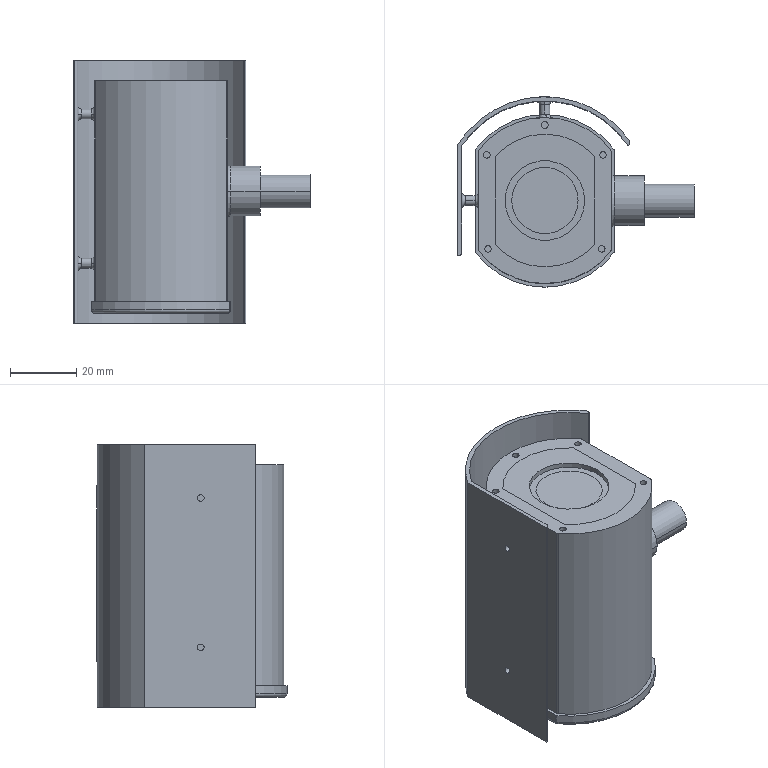Part | SolidWorks | features ICE 17, Dome 1, Extrusion 1, Fillet 1, MirrorSolid 1, Scale 1 | 3 solids | 205 faces | box 71.25 x 57.25 x 79 mm | volume 131185 mm3 | plane 101 | cylinder 78 | torus 12 | spline 8 | sphere 6 | commonest cylinder face diameters 2 x31 3 x12 45 x11 20 x4 24 x4 40 x4